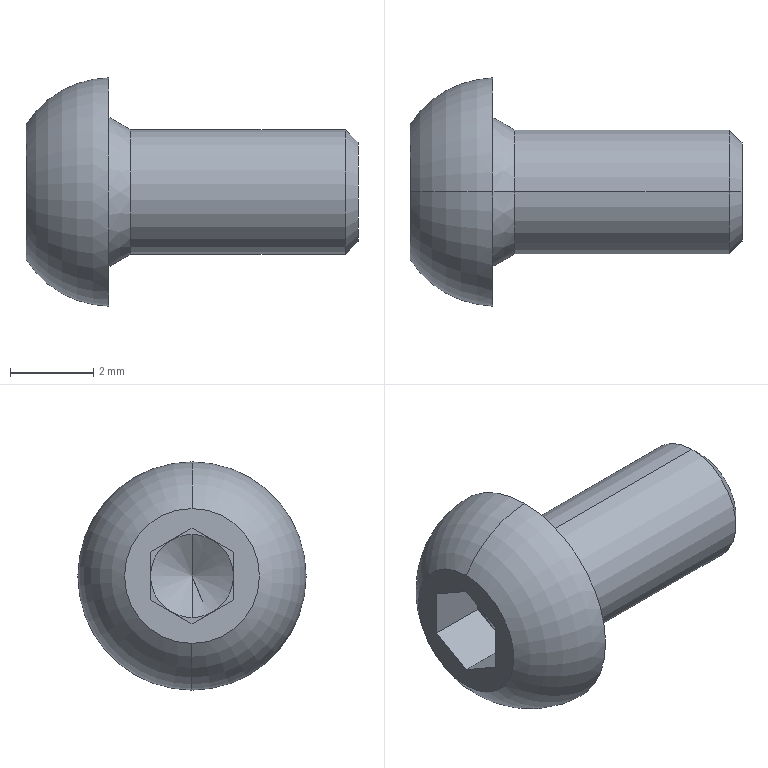Part | NX | features BREP 1 | 1 solid | 25 faces | box 8 x 5.5 x 5.5 mm | volume 74.567 mm3 | plane 15 | cone 6 | cylinder 2 | torus 2 | commonest cylinder face diameters 3 x2
STEP:
#1=CARTESIAN_POINT('',(1.977,0.,0.));
#2=VERTEX_POINT('',#1);
#3=CARTESIAN_POINT('',(1.4,0.,1.));
#4=VERTEX_POINT('',#3);
#5=CARTESIAN_POINT('',(1.4,0.,1.));
#6=DIRECTION('',(-0.5,0.,0.866));
#7=VECTOR('',#6,1000.);
#8=LINE('',#5,#7);
#9=EDGE_CURVE('',#2,#4,#8,.T.);
#10=ORIENTED_EDGE('',*,*,#9,.F.);
#11=CARTESIAN_POINT('',(1.4,0.,-1.));
#12=VERTEX_POINT('',#11);
#13=CARTESIAN_POINT('',(1.4,0.,-1.));
#14=DIRECTION('',(-0.5,0.,-0.866));
#15=VECTOR('',#14,1000.);
#16=LINE('',#13,#15);
#17=EDGE_CURVE('',#2,#12,#16,.T.);
#18=ORIENTED_EDGE('',*,*,#17,.T.);
#19=CARTESIAN_POINT('',(1.4,-0.5,-0.866));
#20=VERTEX_POINT('',#19);
#21=CARTESIAN_POINT('',(1.4,0.,0.));
#22=DIRECTION('',(1.,0.,0.));
#23=DIRECTION('',(0.,0.,1.));
#24=AXIS2_PLACEMENT_3D('',#21,#22,#23);
#25=CIRCLE('',#24,1.);
#26=EDGE_CURVE('',#20,#12,#25,.T.);
#27=ORIENTED_EDGE('',*,*,#26,.F.);
#28=CARTESIAN_POINT('',(1.4,-1.,0.));
#29=VERTEX_POINT('',#28);
#30=CARTESIAN_POINT('',(1.4,0.,0.));
#31=DIRECTION('',(1.,0.,0.));
#32=DIRECTION('',(0.,0.,1.));
#33=AXIS2_PLACEMENT_3D('',#30,#31,#32);
#34=CIRCLE('',#33,1.);
#35=EDGE_CURVE('',#29,#20,#34,.T.);
#36=ORIENTED_EDGE('',*,*,#35,.F.);
#37=CARTESIAN_POINT('',(1.4,-0.5,0.866));
#38=VERTEX_POINT('',#37);
#39=CARTESIAN_POINT('',(1.4,0.,0.));
#40=DIRECTION('',(1.,0.,0.));
#41=DIRECTION('',(0.,0.,1.));
#42=AXIS2_PLACEMENT_3D('',#39,#40,#41);
#43=CIRCLE('',#42,1.);
#44=EDGE_CURVE('',#38,#29,#43,.T.);
#45=ORIENTED_EDGE('',*,*,#44,.F.);
#46=CARTESIAN_POINT('',(1.4,0.,0.));
#47=DIRECTION('',(1.,0.,0.));
#48=DIRECTION('',(0.,0.,1.));
#49=AXIS2_PLACEMENT_3D('',#46,#47,#48);
#50=CIRCLE('',#49,1.);
#51=EDGE_CURVE('',#4,#38,#50,.T.);
#52=ORIENTED_EDGE('',*,*,#51,.F.);
#53=EDGE_LOOP('',(#10,#18,#27,#36,#45,#52));
#54=FACE_BOUND('',#53,.T.);
#55=CARTESIAN_POINT('',(1.4,0.,0.));
#56=DIRECTION('',(-1.,0.,0.));
#57=DIRECTION('',(0.,0.,-1.));
#58=AXIS2_PLACEMENT_3D('',#55,#56,#57);
#59=CONICAL_SURFACE('',#58,1.,1.047);
#60=ADVANCED_FACE('',(#54),#59,.F.);
#61=CARTESIAN_POINT('',(8.,0.,1.194));
#62=VERTEX_POINT('',#61);
#63=CARTESIAN_POINT('',(8.,0.,-1.194));
#64=VERTEX_POINT('',#63);
#65=CARTESIAN_POINT('',(8.,0.,0.));
#66=DIRECTION('',(-1.,0.,0.));
#67=DIRECTION('',(0.,0.,1.));
#68=AXIS2_PLACEMENT_3D('',#65,#66,#67);
#69=CIRCLE('',#68,1.194);
#70=EDGE_CURVE('',#62,#64,#69,.T.);
#71=ORIENTED_EDGE('',*,*,#70,.T.);
#72=CARTESIAN_POINT('',(7.694,0.,-1.5));
#73=VERTEX_POINT('',#72);
#74=CARTESIAN_POINT('',(8.,0.,-1.194));
#75=DIRECTION('',(-0.7071,0.,-0.7071));
#76=VECTOR('',#75,1000.);
#77=LINE('',#74,#76);
#78=EDGE_CURVE('',#64,#73,#77,.T.);
#79=ORIENTED_EDGE('',*,*,#78,.T.);
#80=CARTESIAN_POINT('',(7.694,0.,1.5));
#81=VERTEX_POINT('',#80);
#82=CARTESIAN_POINT('',(7.694,0.,0.));
#83=DIRECTION('',(-1.,0.,0.));
#84=DIRECTION('',(0.,0.,1.));
#85=AXIS2_PLACEMENT_3D('',#82,#83,#84);
#86=CIRCLE('',#85,1.5);
#87=EDGE_CURVE('',#81,#73,#86,.T.);
#88=ORIENTED_EDGE('',*,*,#87,.F.);
#89=CARTESIAN_POINT('',(8.,0.,1.194));
#90=DIRECTION('',(-0.7071,0.,0.7071));
#91=VECTOR('',#90,1000.);
#92=LINE('',#89,#91);
#93=EDGE_CURVE('',#62,#81,#92,.T.);
#94=ORIENTED_EDGE('',*,*,#93,.F.);
#95=EDGE_LOOP('',(#71,#79,#88,#94));
#96=FACE_BOUND('',#95,.T.);
#97=CARTESIAN_POINT('',(8.,0.,0.));
#98=DIRECTION('',(-1.,0.,0.));
#99=DIRECTION('',(0.,0.,-1.));
#100=AXIS2_PLACEMENT_3D('',#97,#98,#99);
#101=CONICAL_SURFACE('',#100,1.194,0.7854);
#102=ADVANCED_FACE('',(#96),#101,.T.);
#103=ORIENTED_EDGE('',*,*,#87,.T.);
#104=CARTESIAN_POINT('',(2.52,0.,-1.5));
#105=VERTEX_POINT('',#104);
#106=CARTESIAN_POINT('',(8.,0.,-1.5));
#107=DIRECTION('',(-1.,0.,0.));
#108=VECTOR('',#107,1000.);
#109=LINE('',#106,#108);
#110=EDGE_CURVE('',#73,#105,#109,.T.);
#111=ORIENTED_EDGE('',*,*,#110,.T.);
#112=CARTESIAN_POINT('',(2.52,0.,1.5));
#113=VERTEX_POINT('',#112);
#114=CARTESIAN_POINT('',(2.52,0.,0.));
#115=DIRECTION('',(-1.,0.,0.));
#116=DIRECTION('',(0.,0.,1.));
#117=AXIS2_PLACEMENT_3D('',#114,#115,#116);
#118=CIRCLE('',#117,1.5);
#119=EDGE_CURVE('',#113,#105,#118,.T.);
#120=ORIENTED_EDGE('',*,*,#119,.F.);
#121=CARTESIAN_POINT('',(8.,0.,1.5));
#122=DIRECTION('',(-1.,0.,0.));
#123=VECTOR('',#122,1000.);
#124=LINE('',#121,#123);
#125=EDGE_CURVE('',#81,#113,#124,.T.);
#126=ORIENTED_EDGE('',*,*,#125,.F.);
#127=EDGE_LOOP('',(#103,#111,#120,#126));
#128=FACE_BOUND('',#127,.T.);
#129=CARTESIAN_POINT('',(8.,0.,0.));
#130=DIRECTION('',(-1.,0.,0.));
#131=DIRECTION('',(0.,0.,-1.));
#132=AXIS2_PLACEMENT_3D('',#129,#130,#131);
#133=CYLINDRICAL_SURFACE('',#132,1.5);
#134=ADVANCED_FACE('',(#128),#133,.T.);
#135=ORIENTED_EDGE('',*,*,#119,.T.);
#136=CARTESIAN_POINT('',(2.,0.,-1.8));
#137=VERTEX_POINT('',#136);
#138=CARTESIAN_POINT('',(2.52,0.,-1.5));
#139=DIRECTION('',(-0.866,0.,-0.5));
#140=VECTOR('',#139,1000.);
#141=LINE('',#138,#140);
#142=EDGE_CURVE('',#105,#137,#141,.T.);
#143=ORIENTED_EDGE('',*,*,#142,.T.);
#144=CARTESIAN_POINT('',(2.,0.,1.8));
#145=VERTEX_POINT('',#144);
#146=CARTESIAN_POINT('',(2.,0.,0.));
#147=DIRECTION('',(-1.,0.,0.));
#148=DIRECTION('',(0.,0.,1.));
#149=AXIS2_PLACEMENT_3D('',#146,#147,#148);
#150=CIRCLE('',#149,1.8);
#151=EDGE_CURVE('',#145,#137,#150,.T.);
#152=ORIENTED_EDGE('',*,*,#151,.F.);
#153=CARTESIAN_POINT('',(2.52,0.,1.5));
#154=DIRECTION('',(-0.866,0.,0.5));
#155=VECTOR('',#154,1000.);
#156=LINE('',#153,#155);
#157=EDGE_CURVE('',#113,#145,#156,.T.);
#158=ORIENTED_EDGE('',*,*,#157,.F.);
#159=EDGE_LOOP('',(#135,#143,#152,#158));
#160=FACE_BOUND('',#159,.T.);
#161=CARTESIAN_POINT('',(2.52,0.,0.));
#162=DIRECTION('',(-1.,0.,0.));
#163=DIRECTION('',(0.,0.,-1.));
#164=AXIS2_PLACEMENT_3D('',#161,#162,#163);
#165=CONICAL_SURFACE('',#164,1.5,0.5236);
#166=ADVANCED_FACE('',(#160),#165,.T.);
#167=CARTESIAN_POINT('',(2.,0.,2.75));
#168=VERTEX_POINT('',#167);
#169=CARTESIAN_POINT('',(2.,0.,-2.75));
#170=VERTEX_POINT('',#169);
#171=CARTESIAN_POINT('',(2.,0.,0.));
#172=DIRECTION('',(-1.,0.,0.));
#173=DIRECTION('',(0.,0.,1.));
#174=AXIS2_PLACEMENT_3D('',#171,#172,#173);
#175=CIRCLE('',#174,2.75);
#176=EDGE_CURVE('',#168,#170,#175,.T.);
#177=ORIENTED_EDGE('',*,*,#176,.T.);
#178=CARTESIAN_POINT('',(0.,0.,-1.625));
#179=VERTEX_POINT('',#178);
#180=CARTESIAN_POINT('',(2.033,0.,-0.3502));
#181=DIRECTION('',(0.,1.,0.));
#182=DIRECTION('',(0.,0.,1.));
#183=AXIS2_PLACEMENT_3D('',#180,#181,#182);
#184=CIRCLE('',#183,2.4);
#185=EDGE_CURVE('',#170,#179,#184,.T.);
#186=ORIENTED_EDGE('',*,*,#185,.T.);
#187=CARTESIAN_POINT('',(0.,0.,1.625));
#188=VERTEX_POINT('',#187);
#189=CARTESIAN_POINT('',(0.,0.,0.));
#190=DIRECTION('',(-1.,0.,0.));
#191=DIRECTION('',(0.,0.,1.));
#192=AXIS2_PLACEMENT_3D('',#189,#190,#191);
#193=CIRCLE('',#192,1.625);
#194=EDGE_CURVE('',#188,#179,#193,.T.);
#195=ORIENTED_EDGE('',*,*,#194,.F.);
#196=CARTESIAN_POINT('',(2.033,0.,0.3502));
#197=DIRECTION('',(0.,-1.,0.));
#198=DIRECTION('',(0.,0.,-1.));
#199=AXIS2_PLACEMENT_3D('',#196,#197,#198);
#200=CIRCLE('',#199,2.4);
#201=EDGE_CURVE('',#168,#188,#200,.T.);
#202=ORIENTED_EDGE('',*,*,#201,.F.);
#203=EDGE_LOOP('',(#177,#186,#195,#202));
#204=FACE_BOUND('',#203,.T.);
#205=CARTESIAN_POINT('',(2.033,0.,0.));
#206=DIRECTION('',(-1.,0.,0.));
#207=DIRECTION('',(0.,0.,-1.));
#208=AXIS2_PLACEMENT_3D('',#205,#206,#207);
#209=DEGENERATE_TOROIDAL_SURFACE('',#208,0.3502,2.4,.T.);
#210=ADVANCED_FACE('',(#204),#209,.T.);
#211=CARTESIAN_POINT('',(0.,-1.,0.5774));
#212=VERTEX_POINT('',#211);
#213=CARTESIAN_POINT('',(0.,0.,1.155));
#214=VERTEX_POINT('',#213);
#215=CARTESIAN_POINT('',(0.,-1.,0.5774));
#216=DIRECTION('',(0.,0.866,0.5));
#217=VECTOR('',#216,1000.);
#218=LINE('',#215,#217);
#219=EDGE_CURVE('',#212,#214,#218,.T.);
#220=ORIENTED_EDGE('',*,*,#219,.F.);
#221=CARTESIAN_POINT('',(0.,-1.,-0.5774));
#222=VERTEX_POINT('',#221);
#223=CARTESIAN_POINT('',(0.,-1.,-0.5774));
#224=DIRECTION('',(0.,0.,1.));
#225=VECTOR('',#224,1000.);
#226=LINE('',#223,#225);
#227=EDGE_CURVE('',#222,#212,#226,.T.);
#228=ORIENTED_EDGE('',*,*,#227,.F.);
#229=CARTESIAN_POINT('',(0.,0.,-1.155));
#230=VERTEX_POINT('',#229);
#231=CARTESIAN_POINT('',(0.,0.,-1.155));
#232=DIRECTION('',(0.,-0.866,0.5));
#233=VECTOR('',#232,1000.);
#234=LINE('',#231,#233);
#235=EDGE_CURVE('',#230,#222,#234,.T.);
#236=ORIENTED_EDGE('',*,*,#235,.F.);
#237=CARTESIAN_POINT('',(0.,1.,-0.5774));
#238=VERTEX_POINT('',#237);
#239=CARTESIAN_POINT('',(0.,1.,-0.5774));
#240=DIRECTION('',(0.,-0.866,-0.5));
#241=VECTOR('',#240,1000.);
#242=LINE('',#239,#241);
#243=EDGE_CURVE('',#238,#230,#242,.T.);
#244=ORIENTED_EDGE('',*,*,#243,.F.);
#245=CARTESIAN_POINT('',(0.,1.,0.5774));
#246=VERTEX_POINT('',#245);
#247=CARTESIAN_POINT('',(0.,1.,0.5774));
#248=DIRECTION('',(0.,0.,-1.));
#249=VECTOR('',#248,1000.);
#250=LINE('',#247,#249);
#251=EDGE_CURVE('',#246,#238,#250,.T.);
#252=ORIENTED_EDGE('',*,*,#251,.F.);
#253=CARTESIAN_POINT('',(0.,0.,1.155));
#254=DIRECTION('',(0.,0.866,-0.5));
#255=VECTOR('',#254,1000.);
#256=LINE('',#253,#255);
#257=EDGE_CURVE('',#214,#246,#256,.T.);
#258=ORIENTED_EDGE('',*,*,#257,.F.);
#259=EDGE_LOOP('',(#220,#228,#236,#244,#252,#258));
#260=FACE_BOUND('',#259,.T.);
#261=ORIENTED_EDGE('',*,*,#194,.T.);
#262=CARTESIAN_POINT('',(0.,0.,0.));
#263=DIRECTION('',(-1.,0.,0.));
#264=DIRECTION('',(0.,0.,1.));
#265=AXIS2_PLACEMENT_3D('',#262,#263,#264);
#266=CIRCLE('',#265,1.625);
#267=EDGE_CURVE('',#179,#188,#266,.T.);
#268=ORIENTED_EDGE('',*,*,#267,.T.);
#269=EDGE_LOOP('',(#261,#268));
#270=FACE_BOUND('',#269,.T.);
#271=CARTESIAN_POINT('',(0.,0.5,0.));
#272=DIRECTION('',(1.,0.,0.));
#273=DIRECTION('',(0.,0.,1.));
#274=AXIS2_PLACEMENT_3D('',#271,#272,#273);
#275=PLANE('',#274);
#276=ADVANCED_FACE('',(#260,#270),#275,.F.);
#277=ORIENTED_EDGE('',*,*,#185,.F.);
#278=CARTESIAN_POINT('',(2.,0.,0.));
#279=DIRECTION('',(-1.,0.,0.));
#280=DIRECTION('',(0.,0.,1.));
#281=AXIS2_PLACEMENT_3D('',#278,#279,#280);
#282=CIRCLE('',#281,2.75);
#283=EDGE_CURVE('',#170,#168,#282,.T.);
#284=ORIENTED_EDGE('',*,*,#283,.T.);
#285=ORIENTED_EDGE('',*,*,#201,.T.);
#286=ORIENTED_EDGE('',*,*,#267,.F.);
#287=EDGE_LOOP('',(#277,#284,#285,#286));
#288=FACE_BOUND('',#287,.T.);
#289=CARTESIAN_POINT('',(2.033,0.,0.));
#290=DIRECTION('',(-1.,0.,0.));
#291=DIRECTION('',(0.,0.,-1.));
#292=AXIS2_PLACEMENT_3D('',#289,#290,#291);
#293=DEGENERATE_TOROIDAL_SURFACE('',#292,0.3502,2.4,.T.);
#294=ADVANCED_FACE('',(#288),#293,.T.);
#295=ORIENTED_EDGE('',*,*,#176,.F.);
#296=ORIENTED_EDGE('',*,*,#283,.F.);
#297=EDGE_LOOP('',(#295,#296));
#298=FACE_BOUND('',#297,.T.);
#299=ORIENTED_EDGE('',*,*,#151,.T.);
#300=CARTESIAN_POINT('',(2.,0.,0.));
#301=DIRECTION('',(-1.,0.,0.));
#302=DIRECTION('',(0.,0.,1.));
#303=AXIS2_PLACEMENT_3D('',#300,#301,#302);
#304=CIRCLE('',#303,1.8);
#305=EDGE_CURVE('',#137,#145,#304,.T.);
#306=ORIENTED_EDGE('',*,*,#305,.T.);
#307=EDGE_LOOP('',(#299,#306));
#308=FACE_BOUND('',#307,.T.);
#309=CARTESIAN_POINT('',(2.,2.75,0.));
#310=DIRECTION('',(-1.,0.,0.));
#311=DIRECTION('',(0.,0.,-1.));
#312=AXIS2_PLACEMENT_3D('',#309,#310,#311);
#313=PLANE('',#312);
#314=ADVANCED_FACE('',(#298,#308),#313,.F.);
#315=ORIENTED_EDGE('',*,*,#142,.F.);
#316=CARTESIAN_POINT('',(2.52,0.,0.));
#317=DIRECTION('',(-1.,0.,0.));
#318=DIRECTION('',(0.,0.,1.));
#319=AXIS2_PLACEMENT_3D('',#316,#317,#318);
#320=CIRCLE('',#319,1.5);
#321=EDGE_CURVE('',#105,#113,#320,.T.);
#322=ORIENTED_EDGE('',*,*,#321,.T.);
#323=ORIENTED_EDGE('',*,*,#157,.T.);
#324=ORIENTED_EDGE('',*,*,#305,.F.);
#325=EDGE_LOOP('',(#315,#322,#323,#324));
#326=FACE_BOUND('',#325,.T.);
#327=CARTESIAN_POINT('',(2.52,0.,0.));
#328=DIRECTION('',(-1.,0.,0.));
#329=DIRECTION('',(0.,0.,-1.));
#330=AXIS2_PLACEMENT_3D('',#327,#328,#329);
#331=CONICAL_SURFACE('',#330,1.5,0.5236);
#332=ADVANCED_FACE('',(#326),#331,.T.);
#333=ORIENTED_EDGE('',*,*,#110,.F.);
#334=CARTESIAN_POINT('',(7.694,0.,0.));
#335=DIRECTION('',(-1.,0.,0.));
#336=DIRECTION('',(0.,0.,1.));
#337=AXIS2_PLACEMENT_3D('',#334,#335,#336);
#338=CIRCLE('',#337,1.5);
#339=EDGE_CURVE('',#73,#81,#338,.T.);
#340=ORIENTED_EDGE('',*,*,#339,.T.);
#341=ORIENTED_EDGE('',*,*,#125,.T.);
#342=ORIENTED_EDGE('',*,*,#321,.F.);
#343=EDGE_LOOP('',(#333,#340,#341,#342));
#344=FACE_BOUND('',#343,.T.);
#345=CARTESIAN_POINT('',(8.,0.,0.));
#346=DIRECTION('',(-1.,0.,0.));
#347=DIRECTION('',(0.,0.,-1.));
#348=AXIS2_PLACEMENT_3D('',#345,#346,#347);
#349=CYLINDRICAL_SURFACE('',#348,1.5);
#350=ADVANCED_FACE('',(#344),#349,.T.);
#351=ORIENTED_EDGE('',*,*,#78,.F.);
#352=CARTESIAN_POINT('',(8.,0.,0.));
#353=DIRECTION('',(-1.,0.,0.));
#354=DIRECTION('',(0.,0.,1.));
#355=AXIS2_PLACEMENT_3D('',#352,#353,#354);
#356=CIRCLE('',#355,1.194);
#357=EDGE_CURVE('',#64,#62,#356,.T.);
#358=ORIENTED_EDGE('',*,*,#357,.T.);
#359=ORIENTED_EDGE('',*,*,#93,.T.);
#360=ORIENTED_EDGE('',*,*,#339,.F.);
#361=EDGE_LOOP('',(#351,#358,#359,#360));
#362=FACE_BOUND('',#361,.T.);
#363=CARTESIAN_POINT('',(8.,0.,0.));
#364=DIRECTION('',(-1.,0.,0.));
#365=DIRECTION('',(0.,0.,-1.));
#366=AXIS2_PLACEMENT_3D('',#363,#364,#365);
#367=CONICAL_SURFACE('',#366,1.194,0.7854);
#368=ADVANCED_FACE('',(#362),#367,.T.);
#369=ORIENTED_EDGE('',*,*,#70,.F.);
#370=ORIENTED_EDGE('',*,*,#357,.F.);
#371=EDGE_LOOP('',(#369,#370));
#372=FACE_BOUND('',#371,.T.);
#373=CARTESIAN_POINT('',(8.,1.194,0.));
#374=DIRECTION('',(-1.,0.,0.));
#375=DIRECTION('',(0.,0.,-1.));
#376=AXIS2_PLACEMENT_3D('',#373,#374,#375);
#377=PLANE('',#376);
#378=ADVANCED_FACE('',(#372),#377,.F.);
#379=ORIENTED_EDGE('',*,*,#44,.T.);
#380=CARTESIAN_POINT('',(1.4,-1.,0.5774));
#381=VERTEX_POINT('',#380);
#382=CARTESIAN_POINT('',(1.4,-1.,-0.5774));
#383=DIRECTION('',(0.,0.,1.));
#384=VECTOR('',#383,1000.);
#385=LINE('',#382,#384);
#386=EDGE_CURVE('',#29,#381,#385,.T.);
#387=ORIENTED_EDGE('',*,*,#386,.T.);
#388=CARTESIAN_POINT('',(1.4,-1.,0.5774));
#389=DIRECTION('',(0.,0.866,0.5));
#390=VECTOR('',#389,1000.);
#391=LINE('',#388,#390);
#392=EDGE_CURVE('',#381,#38,#391,.T.);
#393=ORIENTED_EDGE('',*,*,#392,.T.);
#394=EDGE_LOOP('',(#379,#387,#393));
#395=FACE_BOUND('',#394,.T.);
#396=CARTESIAN_POINT('',(1.4,0.,0.));
#397=DIRECTION('',(-1.,0.,0.));
#398=DIRECTION('',(0.,0.,-1.));
#399=AXIS2_PLACEMENT_3D('',#396,#397,#398);
#400=PLANE('',#399);
#401=ADVANCED_FACE('',(#395),#400,.T.);
#402=ORIENTED_EDGE('',*,*,#35,.T.);
#403=CARTESIAN_POINT('',(1.4,-1.,-0.5774));
#404=VERTEX_POINT('',#403);
#405=CARTESIAN_POINT('',(1.4,0.,-1.155));
#406=DIRECTION('',(0.,-0.866,0.5));
#407=VECTOR('',#406,1000.);
#408=LINE('',#405,#407);
#409=EDGE_CURVE('',#20,#404,#408,.T.);
#410=ORIENTED_EDGE('',*,*,#409,.T.);
#411=CARTESIAN_POINT('',(1.4,-1.,-0.5774));
#412=DIRECTION('',(0.,0.,1.));
#413=VECTOR('',#412,1000.);
#414=LINE('',#411,#413);
#415=EDGE_CURVE('',#404,#29,#414,.T.);
#416=ORIENTED_EDGE('',*,*,#415,.T.);
#417=EDGE_LOOP('',(#402,#410,#416));
#418=FACE_BOUND('',#417,.T.);
#419=CARTESIAN_POINT('',(1.4,0.,0.));
#420=DIRECTION('',(-1.,0.,0.));
#421=DIRECTION('',(0.,0.,-1.));
#422=AXIS2_PLACEMENT_3D('',#419,#420,#421);
#423=PLANE('',#422);
#424=ADVANCED_FACE('',(#418),#423,.T.);
#425=ORIENTED_EDGE('',*,*,#26,.T.);
#426=CARTESIAN_POINT('',(1.4,0.5,-0.866));
#427=VERTEX_POINT('',#426);
#428=CARTESIAN_POINT('',(1.4,0.,0.));
#429=DIRECTION('',(1.,0.,0.));
#430=DIRECTION('',(0.,0.,1.));
#431=AXIS2_PLACEMENT_3D('',#428,#429,#430);
#432=CIRCLE('',#431,1.);
#433=EDGE_CURVE('',#12,#427,#432,.T.);
#434=ORIENTED_EDGE('',*,*,#433,.T.);
#435=CARTESIAN_POINT('',(1.4,0.,-1.155));
#436=VERTEX_POINT('',#435);
#437=CARTESIAN_POINT('',(1.4,1.,-0.5774));
#438=DIRECTION('',(0.,-0.866,-0.5));
#439=VECTOR('',#438,1000.);
#440=LINE('',#437,#439);
#441=EDGE_CURVE('',#427,#436,#440,.T.);
#442=ORIENTED_EDGE('',*,*,#441,.T.);
#443=CARTESIAN_POINT('',(1.4,0.,-1.155));
#444=DIRECTION('',(0.,-0.866,0.5));
#445=VECTOR('',#444,1000.);
#446=LINE('',#443,#445);
#447=EDGE_CURVE('',#436,#20,#446,.T.);
#448=ORIENTED_EDGE('',*,*,#447,.T.);
#449=EDGE_LOOP('',(#425,#434,#442,#448));
#450=FACE_BOUND('',#449,.T.);
#451=CARTESIAN_POINT('',(1.4,0.,0.));
#452=DIRECTION('',(-1.,0.,0.));
#453=DIRECTION('',(0.,0.,-1.));
#454=AXIS2_PLACEMENT_3D('',#451,#452,#453);
#455=PLANE('',#454);
#456=ADVANCED_FACE('',(#450),#455,.T.);
#457=CARTESIAN_POINT('',(1.4,1.,0.));
#458=VERTEX_POINT('',#457);
#459=CARTESIAN_POINT('',(1.4,0.,0.));
#460=DIRECTION('',(1.,0.,0.));
#461=DIRECTION('',(0.,0.,1.));
#462=AXIS2_PLACEMENT_3D('',#459,#460,#461);
#463=CIRCLE('',#462,1.);
#464=EDGE_CURVE('',#427,#458,#463,.T.);
#465=ORIENTED_EDGE('',*,*,#464,.T.);
#466=CARTESIAN_POINT('',(1.4,1.,-0.5774));
#467=VERTEX_POINT('',#466);
#468=CARTESIAN_POINT('',(1.4,1.,0.5774));
#469=DIRECTION('',(0.,0.,-1.));
#470=VECTOR('',#469,1000.);
#471=LINE('',#468,#470);
#472=EDGE_CURVE('',#458,#467,#471,.T.);
#473=ORIENTED_EDGE('',*,*,#472,.T.);
#474=CARTESIAN_POINT('',(1.4,1.,-0.5774));
#475=DIRECTION('',(0.,-0.866,-0.5));
#476=VECTOR('',#475,1000.);
#477=LINE('',#474,#476);
#478=EDGE_CURVE('',#467,#427,#477,.T.);
#479=ORIENTED_EDGE('',*,*,#478,.T.);
#480=EDGE_LOOP('',(#465,#473,#479));
#481=FACE_BOUND('',#480,.T.);
#482=CARTESIAN_POINT('',(1.4,0.,0.));
#483=DIRECTION('',(-1.,0.,0.));
#484=DIRECTION('',(0.,0.,-1.));
#485=AXIS2_PLACEMENT_3D('',#482,#483,#484);
#486=PLANE('',#485);
#487=ADVANCED_FACE('',(#481),#486,.T.);
#488=CARTESIAN_POINT('',(1.4,0.5,0.866));
#489=VERTEX_POINT('',#488);
#490=CARTESIAN_POINT('',(1.4,0.,0.));
#491=DIRECTION('',(-1.,0.,0.));
#492=DIRECTION('',(0.,0.,1.));
#493=AXIS2_PLACEMENT_3D('',#490,#491,#492);
#494=CIRCLE('',#493,1.);
#495=EDGE_CURVE('',#489,#458,#494,.T.);
#496=ORIENTED_EDGE('',*,*,#495,.F.);
#497=CARTESIAN_POINT('',(1.4,1.,0.5774));
#498=VERTEX_POINT('',#497);
#499=CARTESIAN_POINT('',(1.4,0.,1.155));
#500=DIRECTION('',(0.,0.866,-0.5));
#501=VECTOR('',#500,1000.);
#502=LINE('',#499,#501);
#503=EDGE_CURVE('',#489,#498,#502,.T.);
#504=ORIENTED_EDGE('',*,*,#503,.T.);
#505=CARTESIAN_POINT('',(1.4,1.,0.5774));
#506=DIRECTION('',(0.,0.,-1.));
#507=VECTOR('',#506,1000.);
#508=LINE('',#505,#507);
#509=EDGE_CURVE('',#498,#458,#508,.T.);
#510=ORIENTED_EDGE('',*,*,#509,.T.);
#511=EDGE_LOOP('',(#496,#504,#510));
#512=FACE_BOUND('',#511,.T.);
#513=CARTESIAN_POINT('',(1.4,0.,0.));
#514=DIRECTION('',(-1.,0.,0.));
#515=DIRECTION('',(0.,0.,-1.));
#516=AXIS2_PLACEMENT_3D('',#513,#514,#515);
#517=PLANE('',#516);
#518=ADVANCED_FACE('',(#512),#517,.T.);
#519=CARTESIAN_POINT('',(1.4,0.,0.));
#520=DIRECTION('',(1.,0.,0.));
#521=DIRECTION('',(0.,0.,1.));
#522=AXIS2_PLACEMENT_3D('',#519,#520,#521);
#523=CIRCLE('',#522,1.);
#524=EDGE_CURVE('',#489,#4,#523,.T.);
#525=ORIENTED_EDGE('',*,*,#524,.T.);
#526=ORIENTED_EDGE('',*,*,#51,.T.);
#527=CARTESIAN_POINT('',(1.4,0.,1.155));
#528=VERTEX_POINT('',#527);
#529=CARTESIAN_POINT('',(1.4,-1.,0.5774));
#530=DIRECTION('',(0.,0.866,0.5));
#531=VECTOR('',#530,1000.);
#532=LINE('',#529,#531);
#533=EDGE_CURVE('',#38,#528,#532,.T.);
#534=ORIENTED_EDGE('',*,*,#533,.T.);
#535=CARTESIAN_POINT('',(1.4,0.,1.155));
#536=DIRECTION('',(0.,0.866,-0.5));
#537=VECTOR('',#536,1000.);
#538=LINE('',#535,#537);
#539=EDGE_CURVE('',#528,#489,#538,.T.);
#540=ORIENTED_EDGE('',*,*,#539,.T.);
#541=EDGE_LOOP('',(#525,#526,#534,#540));
#542=FACE_BOUND('',#541,.T.);
#543=CARTESIAN_POINT('',(1.4,0.,0.));
#544=DIRECTION('',(-1.,0.,0.));
#545=DIRECTION('',(0.,0.,-1.));
#546=AXIS2_PLACEMENT_3D('',#543,#544,#545);
#547=PLANE('',#546);
#548=ADVANCED_FACE('',(#542),#547,.T.);
#549=ORIENTED_EDGE('',*,*,#227,.T.);
#550=CARTESIAN_POINT('',(1.4,-1.,0.5774));
#551=DIRECTION('',(-1.,0.,0.));
#552=VECTOR('',#551,1000.);
#553=LINE('',#550,#552);
#554=EDGE_CURVE('',#381,#212,#553,.T.);
#555=ORIENTED_EDGE('',*,*,#554,.F.);
#556=ORIENTED_EDGE('',*,*,#386,.F.);
#557=ORIENTED_EDGE('',*,*,#415,.F.);
#558=CARTESIAN_POINT('',(1.4,-1.,-0.5774));
#559=DIRECTION('',(-1.,0.,0.));
#560=VECTOR('',#559,1000.);
#561=LINE('',#558,#560);
#562=EDGE_CURVE('',#404,#222,#561,.T.);
#563=ORIENTED_EDGE('',*,*,#562,.T.);
#564=EDGE_LOOP('',(#549,#555,#556,#557,#563));
#565=FACE_BOUND('',#564,.T.);
#566=CARTESIAN_POINT('',(1.4,-1.,-0.5774));
#567=DIRECTION('',(0.,-1.,0.));
#568=DIRECTION('',(0.,0.,1.));
#569=AXIS2_PLACEMENT_3D('',#566,#567,#568);
#570=PLANE('',#569);
#571=ADVANCED_FACE('',(#565),#570,.F.);
#572=ORIENTED_EDGE('',*,*,#235,.T.);
#573=ORIENTED_EDGE('',*,*,#562,.F.);
#574=ORIENTED_EDGE('',*,*,#409,.F.);
#575=ORIENTED_EDGE('',*,*,#447,.F.);
#576=CARTESIAN_POINT('',(1.4,0.,-1.155));
#577=DIRECTION('',(-1.,0.,0.));
#578=VECTOR('',#577,1000.);
#579=LINE('',#576,#578);
#580=EDGE_CURVE('',#436,#230,#579,.T.);
#581=ORIENTED_EDGE('',*,*,#580,.T.);
#582=EDGE_LOOP('',(#572,#573,#574,#575,#581));
#583=FACE_BOUND('',#582,.T.);
#584=CARTESIAN_POINT('',(1.4,0.,-1.155));
#585=DIRECTION('',(0.,-0.5,-0.866));
#586=DIRECTION('',(0.,-0.866,0.5));
#587=AXIS2_PLACEMENT_3D('',#584,#585,#586);
#588=PLANE('',#587);
#589=ADVANCED_FACE('',(#583),#588,.F.);
#590=ORIENTED_EDGE('',*,*,#243,.T.);
#591=ORIENTED_EDGE('',*,*,#580,.F.);
#592=ORIENTED_EDGE('',*,*,#441,.F.);
#593=ORIENTED_EDGE('',*,*,#478,.F.);
#594=CARTESIAN_POINT('',(1.4,1.,-0.5774));
#595=DIRECTION('',(-1.,0.,0.));
#596=VECTOR('',#595,1000.);
#597=LINE('',#594,#596);
#598=EDGE_CURVE('',#467,#238,#597,.T.);
#599=ORIENTED_EDGE('',*,*,#598,.T.);
#600=EDGE_LOOP('',(#590,#591,#592,#593,#599));
#601=FACE_BOUND('',#600,.T.);
#602=CARTESIAN_POINT('',(1.4,1.,-0.5774));
#603=DIRECTION('',(0.,0.5,-0.866));
#604=DIRECTION('',(0.,-0.866,-0.5));
#605=AXIS2_PLACEMENT_3D('',#602,#603,#604);
#606=PLANE('',#605);
#607=ADVANCED_FACE('',(#601),#606,.F.);
#608=ORIENTED_EDGE('',*,*,#251,.T.);
#609=ORIENTED_EDGE('',*,*,#598,.F.);
#610=ORIENTED_EDGE('',*,*,#472,.F.);
#611=ORIENTED_EDGE('',*,*,#509,.F.);
#612=CARTESIAN_POINT('',(1.4,1.,0.5774));
#613=DIRECTION('',(-1.,0.,0.));
#614=VECTOR('',#613,1000.);
#615=LINE('',#612,#614);
#616=EDGE_CURVE('',#498,#246,#615,.T.);
#617=ORIENTED_EDGE('',*,*,#616,.T.);
#618=EDGE_LOOP('',(#608,#609,#610,#611,#617));
#619=FACE_BOUND('',#618,.T.);
#620=CARTESIAN_POINT('',(1.4,1.,0.5774));
#621=DIRECTION('',(0.,1.,0.));
#622=DIRECTION('',(0.,0.,-1.));
#623=AXIS2_PLACEMENT_3D('',#620,#621,#622);
#624=PLANE('',#623);
#625=ADVANCED_FACE('',(#619),#624,.F.);
#626=ORIENTED_EDGE('',*,*,#257,.T.);
#627=ORIENTED_EDGE('',*,*,#616,.F.);
#628=ORIENTED_EDGE('',*,*,#503,.F.);
#629=ORIENTED_EDGE('',*,*,#539,.F.);
#630=CARTESIAN_POINT('',(1.4,0.,1.155));
#631=DIRECTION('',(-1.,0.,0.));
#632=VECTOR('',#631,1000.);
#633=LINE('',#630,#632);
#634=EDGE_CURVE('',#528,#214,#633,.T.);
#635=ORIENTED_EDGE('',*,*,#634,.T.);
#636=EDGE_LOOP('',(#626,#627,#628,#629,#635));
#637=FACE_BOUND('',#636,.T.);
#638=CARTESIAN_POINT('',(1.4,0.,1.155));
#639=DIRECTION('',(0.,0.5,0.866));
#640=DIRECTION('',(0.,0.866,-0.5));
#641=AXIS2_PLACEMENT_3D('',#638,#639,#640);
#642=PLANE('',#641);
#643=ADVANCED_FACE('',(#637),#642,.F.);
#644=ORIENTED_EDGE('',*,*,#219,.T.);
#645=ORIENTED_EDGE('',*,*,#634,.F.);
#646=ORIENTED_EDGE('',*,*,#533,.F.);
#647=ORIENTED_EDGE('',*,*,#392,.F.);
#648=ORIENTED_EDGE('',*,*,#554,.T.);
#649=EDGE_LOOP('',(#644,#645,#646,#647,#648));
#650=FACE_BOUND('',#649,.T.);
#651=CARTESIAN_POINT('',(1.4,-1.,0.5774));
#652=DIRECTION('',(0.,-0.5,0.866));
#653=DIRECTION('',(0.,0.866,0.5));
#654=AXIS2_PLACEMENT_3D('',#651,#652,#653);
#655=PLANE('',#654);
#656=ADVANCED_FACE('',(#650),#655,.F.);
#657=ORIENTED_EDGE('',*,*,#17,.F.);
#658=ORIENTED_EDGE('',*,*,#9,.T.);
#659=ORIENTED_EDGE('',*,*,#524,.F.);
#660=ORIENTED_EDGE('',*,*,#495,.T.);
#661=ORIENTED_EDGE('',*,*,#464,.F.);
#662=ORIENTED_EDGE('',*,*,#433,.F.);
#663=EDGE_LOOP('',(#657,#658,#659,#660,#661,#662));
#664=FACE_BOUND('',#663,.T.);
#665=CARTESIAN_POINT('',(1.4,0.,0.));
#666=DIRECTION('',(-1.,0.,0.));
#667=DIRECTION('',(0.,0.,-1.));
#668=AXIS2_PLACEMENT_3D('',#665,#666,#667);
#669=CONICAL_SURFACE('',#668,1.,1.047);
#670=ADVANCED_FACE('',(#664),#669,.F.);
#671=CLOSED_SHELL('',(#60,#102,#134,#166,#210,#276,#294,#314,#332,#350,#368,#378,#401,#424,#456,#487,#518,#548,#571,#589,#607,#625,#643,#656,#670));
#672=MANIFOLD_SOLID_BREP('',#671);
#673=(LENGTH_UNIT()NAMED_UNIT(*)SI_UNIT(.MILLI.,.METRE.));
#674=UNCERTAINTY_MEASURE_WITH_UNIT(LENGTH_MEASURE(0.00001),#673,'','');
#675=(NAMED_UNIT(*)PLANE_ANGLE_UNIT()SI_UNIT($,.RADIAN.));
#676=(NAMED_UNIT(*)SI_UNIT($,.STERADIAN.)SOLID_ANGLE_UNIT());
#677=(GEOMETRIC_REPRESENTATION_CONTEXT(3)GLOBAL_UNCERTAINTY_ASSIGNED_CONTEXT((#674))GLOBAL_UNIT_ASSIGNED_CONTEXT((#673,#675,#676))REPRESENTATION_CONTEXT('',''));
#678=ADVANCED_BREP_SHAPE_REPRESENTATION('',(#672),#677);